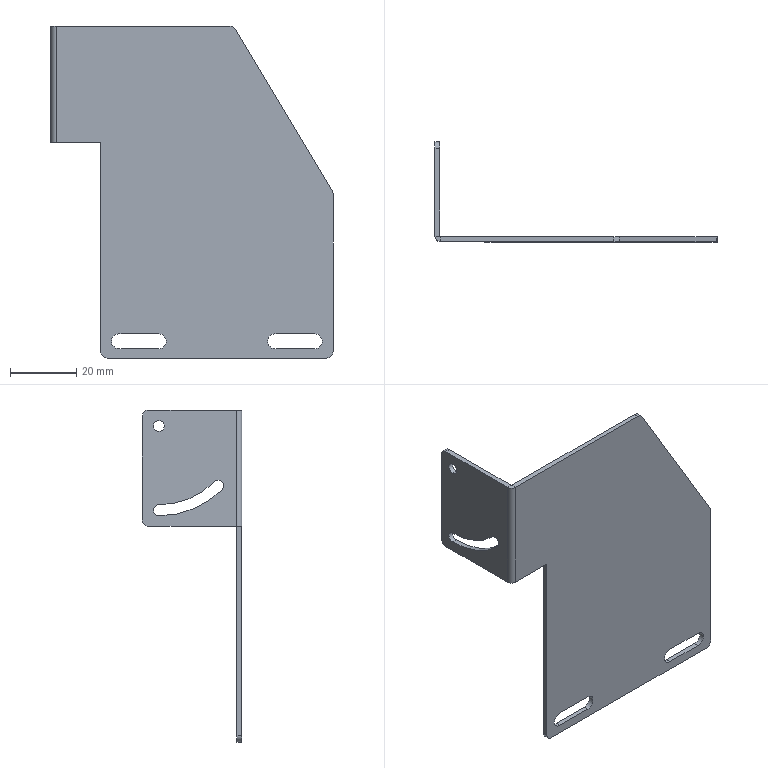Part | STEP file | photoelectric fixing plate 2 | 1 solid | 38 faces | box 85 x 30 x 100 mm | volume 11300 mm3 | cylinder 19 | plane 19 | commonest cylinder face diameters 4 x6 3.3 x5 4.5 x4 0.2 x1 3.2 x1 47.5 x1